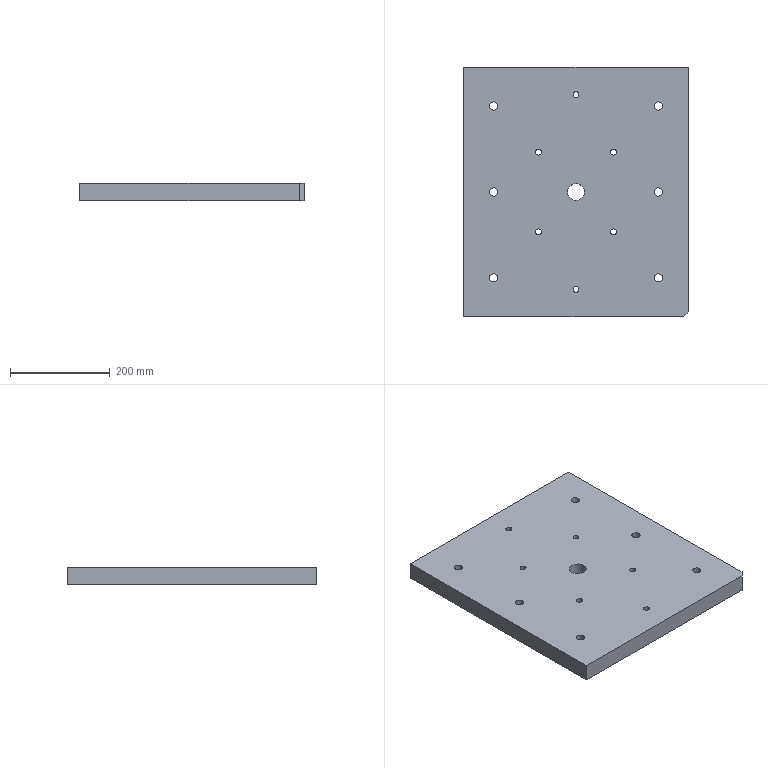Part | STEP file | SL2-MOLD_id750_xmt_txt | 1 solid | 45 faces | box 450 x 500 x 35 mm | volume 7734159 mm3 | cylinder 25 | plane 19 | cone 1 | commonest cylinder face diameters 12 x6 16.5 x6 18 x6 25 x6 34 x1
STEP:
#1=CARTESIAN_POINT('',(225.,340.,-244.));
#2=VERTEX_POINT('',#1);
#3=CARTESIAN_POINT('',(-225.,340.,-244.));
#4=VERTEX_POINT('',#3);
#5=CARTESIAN_POINT('',(0.,340.,-244.));
#6=DIRECTION('',(-1.,0.,0.));
#7=VECTOR('',#6,1.);
#8=LINE('',#5,#7);
#9=EDGE_CURVE('',#2,#4,#8,.T.);
#10=ORIENTED_EDGE('',*,*,#9,.F.);
#11=CARTESIAN_POINT('',(225.,340.,-279.));
#12=VERTEX_POINT('',#11);
#13=CARTESIAN_POINT('',(225.,340.,186.));
#14=DIRECTION('',(0.,0.,1.));
#15=VECTOR('',#14,1.);
#16=LINE('',#13,#15);
#17=EDGE_CURVE('',#12,#2,#16,.T.);
#18=ORIENTED_EDGE('',*,*,#17,.F.);
#19=CARTESIAN_POINT('',(-225.,340.,-279.));
#20=VERTEX_POINT('',#19);
#21=CARTESIAN_POINT('',(0.,340.,-279.));
#22=DIRECTION('',(-1.,0.,0.));
#23=VECTOR('',#22,1.);
#24=LINE('',#21,#23);
#25=EDGE_CURVE('',#12,#20,#24,.T.);
#26=ORIENTED_EDGE('',*,*,#25,.T.);
#27=CARTESIAN_POINT('',(-225.,340.,-279.));
#28=DIRECTION('',(0.,0.,1.));
#29=VECTOR('',#28,1.);
#30=LINE('',#27,#29);
#31=EDGE_CURVE('',#20,#4,#30,.T.);
#32=ORIENTED_EDGE('',*,*,#31,.T.);
#33=EDGE_LOOP('',(#10,#18,#26,#32));
#34=FACE_OUTER_BOUND('',#33,.T.);
#35=CARTESIAN_POINT('',(0.,340.,-279.));
#36=DIRECTION('',(0.,1.,0.));
#37=DIRECTION('',(0.,0.,1.));
#38=AXIS2_PLACEMENT_3D('',#35,#36,#37);
#39=PLANE('',#38);
#40=ADVANCED_FACE('',(#34),#39,.T.);
#41=CARTESIAN_POINT('',(225.,-150.,-244.));
#42=VERTEX_POINT('',#41);
#43=CARTESIAN_POINT('',(225.,0.,-244.));
#44=DIRECTION('',(0.,1.,0.));
#45=VECTOR('',#44,1.);
#46=LINE('',#43,#45);
#47=EDGE_CURVE('',#42,#2,#46,.T.);
#48=ORIENTED_EDGE('',*,*,#47,.F.);
#49=CARTESIAN_POINT('',(225.,-150.,-279.));
#50=VERTEX_POINT('',#49);
#51=CARTESIAN_POINT('',(225.,-150.,186.));
#52=DIRECTION('',(0.,0.,-1.));
#53=VECTOR('',#52,1.);
#54=LINE('',#51,#53);
#55=EDGE_CURVE('',#42,#50,#54,.T.);
#56=ORIENTED_EDGE('',*,*,#55,.T.);
#57=CARTESIAN_POINT('',(225.,0.,-279.));
#58=DIRECTION('',(0.,1.,0.));
#59=VECTOR('',#58,1.);
#60=LINE('',#57,#59);
#61=EDGE_CURVE('',#50,#12,#60,.T.);
#62=ORIENTED_EDGE('',*,*,#61,.T.);
#63=ORIENTED_EDGE('',*,*,#17,.T.);
#64=EDGE_LOOP('',(#48,#56,#62,#63));
#65=FACE_OUTER_BOUND('',#64,.T.);
#66=CARTESIAN_POINT('',(225.,-110.,186.));
#67=DIRECTION('',(1.,0.,0.));
#68=DIRECTION('',(0.,0.,-1.));
#69=AXIS2_PLACEMENT_3D('',#66,#67,#68);
#70=PLANE('',#69);
#71=ADVANCED_FACE('',(#65),#70,.T.);
#72=CARTESIAN_POINT('',(-225.,-160.,-279.));
#73=VERTEX_POINT('',#72);
#74=CARTESIAN_POINT('',(215.,-160.,-279.));
#75=VERTEX_POINT('',#74);
#76=CARTESIAN_POINT('',(0.,-160.,-279.));
#77=DIRECTION('',(1.,0.,0.));
#78=VECTOR('',#77,1.);
#79=LINE('',#76,#78);
#80=EDGE_CURVE('',#73,#75,#79,.T.);
#81=ORIENTED_EDGE('',*,*,#80,.T.);
#82=CARTESIAN_POINT('',(215.,-160.,-244.));
#83=VERTEX_POINT('',#82);
#84=CARTESIAN_POINT('',(215.,-160.,-279.));
#85=DIRECTION('',(0.,0.,1.));
#86=VECTOR('',#85,1.);
#87=LINE('',#84,#86);
#88=EDGE_CURVE('',#75,#83,#87,.T.);
#89=ORIENTED_EDGE('',*,*,#88,.T.);
#90=CARTESIAN_POINT('',(-225.,-160.,-244.));
#91=VERTEX_POINT('',#90);
#92=CARTESIAN_POINT('',(0.,-160.,-244.));
#93=DIRECTION('',(1.,0.,0.));
#94=VECTOR('',#93,1.);
#95=LINE('',#92,#94);
#96=EDGE_CURVE('',#91,#83,#95,.T.);
#97=ORIENTED_EDGE('',*,*,#96,.F.);
#98=CARTESIAN_POINT('',(-225.,-160.,186.));
#99=DIRECTION('',(0.,0.,1.));
#100=VECTOR('',#99,1.);
#101=LINE('',#98,#100);
#102=EDGE_CURVE('',#73,#91,#101,.T.);
#103=ORIENTED_EDGE('',*,*,#102,.F.);
#104=EDGE_LOOP('',(#81,#89,#97,#103));
#105=FACE_OUTER_BOUND('',#104,.T.);
#106=CARTESIAN_POINT('',(0.,-160.,-279.));
#107=DIRECTION('',(0.,-1.,0.));
#108=DIRECTION('',(0.,0.,-1.));
#109=AXIS2_PLACEMENT_3D('',#106,#107,#108);
#110=PLANE('',#109);
#111=ADVANCED_FACE('',(#105),#110,.T.);
#112=CARTESIAN_POINT('',(-225.,0.,-244.));
#113=DIRECTION('',(0.,-1.,0.));
#114=VECTOR('',#113,1.);
#115=LINE('',#112,#114);
#116=EDGE_CURVE('',#4,#91,#115,.T.);
#117=ORIENTED_EDGE('',*,*,#116,.F.);
#118=ORIENTED_EDGE('',*,*,#31,.F.);
#119=CARTESIAN_POINT('',(-225.,0.,-279.));
#120=DIRECTION('',(0.,-1.,0.));
#121=VECTOR('',#120,1.);
#122=LINE('',#119,#121);
#123=EDGE_CURVE('',#20,#73,#122,.T.);
#124=ORIENTED_EDGE('',*,*,#123,.T.);
#125=ORIENTED_EDGE('',*,*,#102,.T.);
#126=EDGE_LOOP('',(#117,#118,#124,#125));
#127=FACE_OUTER_BOUND('',#126,.T.);
#128=CARTESIAN_POINT('',(-225.,-4.582,186.));
#129=DIRECTION('',(-1.,0.,0.));
#130=DIRECTION('',(0.,0.,1.));
#131=AXIS2_PLACEMENT_3D('',#128,#129,#130);
#132=PLANE('',#131);
#133=ADVANCED_FACE('',(#127),#132,.T.);
#134=CARTESIAN_POINT('',(9.,285.,-279.));
#135=VERTEX_POINT('',#134);
#136=CARTESIAN_POINT('',(0.,285.,-279.));
#137=DIRECTION('',(0.,0.,1.));
#138=DIRECTION('',(1.,0.,0.));
#139=AXIS2_PLACEMENT_3D('',#136,#137,#138);
#140=CIRCLE('',#139,9.);
#141=EDGE_CURVE('',#135,#135,#140,.T.);
#142=ORIENTED_EDGE('',*,*,#141,.T.);
#143=EDGE_LOOP('',(#142));
#144=FACE_BOUND('',#143,.T.);
#145=CARTESIAN_POINT('',(84.,170.,-279.));
#146=VERTEX_POINT('',#145);
#147=CARTESIAN_POINT('',(75.,170.,-279.));
#148=DIRECTION('',(0.,0.,1.));
#149=DIRECTION('',(1.,0.,0.));
#150=AXIS2_PLACEMENT_3D('',#147,#148,#149);
#151=CIRCLE('',#150,9.);
#152=EDGE_CURVE('',#146,#146,#151,.T.);
#153=ORIENTED_EDGE('',*,*,#152,.T.);
#154=EDGE_LOOP('',(#153));
#155=FACE_BOUND('',#154,.T.);
#156=CARTESIAN_POINT('',(-66.,170.,-279.));
#157=VERTEX_POINT('',#156);
#158=CARTESIAN_POINT('',(-75.,170.,-279.));
#159=DIRECTION('',(0.,0.,1.));
#160=DIRECTION('',(1.,0.,0.));
#161=AXIS2_PLACEMENT_3D('',#158,#159,#160);
#162=CIRCLE('',#161,9.);
#163=EDGE_CURVE('',#157,#157,#162,.T.);
#164=ORIENTED_EDGE('',*,*,#163,.T.);
#165=EDGE_LOOP('',(#164));
#166=FACE_BOUND('',#165,.T.);
#167=CARTESIAN_POINT('',(-66.,10.,-279.));
#168=VERTEX_POINT('',#167);
#169=CARTESIAN_POINT('',(-75.,10.,-279.));
#170=DIRECTION('',(0.,0.,1.));
#171=DIRECTION('',(1.,0.,0.));
#172=AXIS2_PLACEMENT_3D('',#169,#170,#171);
#173=CIRCLE('',#172,9.);
#174=EDGE_CURVE('',#168,#168,#173,.T.);
#175=ORIENTED_EDGE('',*,*,#174,.T.);
#176=EDGE_LOOP('',(#175));
#177=FACE_BOUND('',#176,.T.);
#178=CARTESIAN_POINT('',(9.,-105.,-279.));
#179=VERTEX_POINT('',#178);
#180=CARTESIAN_POINT('',(0.,-105.,-279.));
#181=DIRECTION('',(0.,0.,1.));
#182=DIRECTION('',(1.,0.,0.));
#183=AXIS2_PLACEMENT_3D('',#180,#181,#182);
#184=CIRCLE('',#183,9.);
#185=EDGE_CURVE('',#179,#179,#184,.T.);
#186=ORIENTED_EDGE('',*,*,#185,.T.);
#187=EDGE_LOOP('',(#186));
#188=FACE_BOUND('',#187,.T.);
#189=CARTESIAN_POINT('',(84.,10.,-279.));
#190=VERTEX_POINT('',#189);
#191=CARTESIAN_POINT('',(75.,10.,-279.));
#192=DIRECTION('',(0.,0.,1.));
#193=DIRECTION('',(1.,0.,0.));
#194=AXIS2_PLACEMENT_3D('',#191,#192,#193);
#195=CIRCLE('',#194,9.);
#196=EDGE_CURVE('',#190,#190,#195,.T.);
#197=ORIENTED_EDGE('',*,*,#196,.T.);
#198=EDGE_LOOP('',(#197));
#199=FACE_BOUND('',#198,.T.);
#200=CARTESIAN_POINT('',(19.,90.,-279.));
#201=VERTEX_POINT('',#200);
#202=CARTESIAN_POINT('',(0.,90.,-279.));
#203=DIRECTION('',(0.,0.,1.));
#204=DIRECTION('',(1.,0.,0.));
#205=AXIS2_PLACEMENT_3D('',#202,#203,#204);
#206=CIRCLE('',#205,19.);
#207=EDGE_CURVE('',#201,#201,#206,.T.);
#208=ORIENTED_EDGE('',*,*,#207,.T.);
#209=EDGE_LOOP('',(#208));
#210=FACE_BOUND('',#209,.T.);
#211=CARTESIAN_POINT('',(177.5,-82.,-279.));
#212=VERTEX_POINT('',#211);
#213=CARTESIAN_POINT('',(165.,-82.,-279.));
#214=DIRECTION('',(0.,0.,-1.));
#215=DIRECTION('',(1.,0.,0.));
#216=AXIS2_PLACEMENT_3D('',#213,#214,#215);
#217=CIRCLE('',#216,12.5);
#218=EDGE_CURVE('',#212,#212,#217,.T.);
#219=ORIENTED_EDGE('',*,*,#218,.F.);
#220=EDGE_LOOP('',(#219));
#221=FACE_BOUND('',#220,.T.);
#222=CARTESIAN_POINT('',(177.5,90.,-279.));
#223=VERTEX_POINT('',#222);
#224=CARTESIAN_POINT('',(165.,90.,-279.));
#225=DIRECTION('',(0.,0.,-1.));
#226=DIRECTION('',(1.,0.,0.));
#227=AXIS2_PLACEMENT_3D('',#224,#225,#226);
#228=CIRCLE('',#227,12.5);
#229=EDGE_CURVE('',#223,#223,#228,.T.);
#230=ORIENTED_EDGE('',*,*,#229,.F.);
#231=EDGE_LOOP('',(#230));
#232=FACE_BOUND('',#231,.T.);
#233=CARTESIAN_POINT('',(-152.5,-82.,-279.));
#234=VERTEX_POINT('',#233);
#235=CARTESIAN_POINT('',(-165.,-82.,-279.));
#236=DIRECTION('',(0.,0.,-1.));
#237=DIRECTION('',(1.,0.,0.));
#238=AXIS2_PLACEMENT_3D('',#235,#236,#237);
#239=CIRCLE('',#238,12.5);
#240=EDGE_CURVE('',#234,#234,#239,.T.);
#241=ORIENTED_EDGE('',*,*,#240,.F.);
#242=EDGE_LOOP('',(#241));
#243=FACE_BOUND('',#242,.T.);
#244=CARTESIAN_POINT('',(-152.5,90.,-279.));
#245=VERTEX_POINT('',#244);
#246=CARTESIAN_POINT('',(-165.,90.,-279.));
#247=DIRECTION('',(0.,0.,-1.));
#248=DIRECTION('',(1.,0.,0.));
#249=AXIS2_PLACEMENT_3D('',#246,#247,#248);
#250=CIRCLE('',#249,12.5);
#251=EDGE_CURVE('',#245,#245,#250,.T.);
#252=ORIENTED_EDGE('',*,*,#251,.F.);
#253=EDGE_LOOP('',(#252));
#254=FACE_BOUND('',#253,.T.);
#255=CARTESIAN_POINT('',(-152.5,262.,-279.));
#256=VERTEX_POINT('',#255);
#257=CARTESIAN_POINT('',(-165.,262.,-279.));
#258=DIRECTION('',(0.,0.,-1.));
#259=DIRECTION('',(1.,0.,0.));
#260=AXIS2_PLACEMENT_3D('',#257,#258,#259);
#261=CIRCLE('',#260,12.5);
#262=EDGE_CURVE('',#256,#256,#261,.T.);
#263=ORIENTED_EDGE('',*,*,#262,.F.);
#264=EDGE_LOOP('',(#263));
#265=FACE_BOUND('',#264,.T.);
#266=CARTESIAN_POINT('',(177.5,262.,-279.));
#267=VERTEX_POINT('',#266);
#268=CARTESIAN_POINT('',(165.,262.,-279.));
#269=DIRECTION('',(0.,0.,-1.));
#270=DIRECTION('',(1.,0.,0.));
#271=AXIS2_PLACEMENT_3D('',#268,#269,#270);
#272=CIRCLE('',#271,12.5);
#273=EDGE_CURVE('',#267,#267,#272,.T.);
#274=ORIENTED_EDGE('',*,*,#273,.F.);
#275=EDGE_LOOP('',(#274));
#276=FACE_BOUND('',#275,.T.);
#277=ORIENTED_EDGE('',*,*,#61,.F.);
#278=CARTESIAN_POINT('',(215.,-160.,-279.));
#279=DIRECTION('',(-0.7071,-0.7071,0.));
#280=VECTOR('',#279,1.);
#281=LINE('',#278,#280);
#282=EDGE_CURVE('',#50,#75,#281,.T.);
#283=ORIENTED_EDGE('',*,*,#282,.T.);
#284=ORIENTED_EDGE('',*,*,#80,.F.);
#285=ORIENTED_EDGE('',*,*,#123,.F.);
#286=ORIENTED_EDGE('',*,*,#25,.F.);
#287=EDGE_LOOP('',(#277,#283,#284,#285,#286));
#288=FACE_BOUND('',#287,.T.);
#289=CARTESIAN_POINT('',(0.,0.,-279.));
#290=DIRECTION('',(0.,0.,1.));
#291=DIRECTION('',(1.,0.,0.));
#292=AXIS2_PLACEMENT_3D('',#289,#290,#291);
#293=PLANE('',#292);
#294=ADVANCED_FACE('',(#144,#155,#166,#177,#188,#199,#210,#221,#232,#243,#254,#265,#276,#288),#293,.F.);
#295=CARTESIAN_POINT('',(-69.,10.,-244.));
#296=VERTEX_POINT('',#295);
#297=CARTESIAN_POINT('',(-75.,10.,-244.));
#298=DIRECTION('',(0.,0.,-1.));
#299=DIRECTION('',(1.,0.,0.));
#300=AXIS2_PLACEMENT_3D('',#297,#298,#299);
#301=CIRCLE('',#300,6.);
#302=EDGE_CURVE('',#296,#296,#301,.T.);
#303=ORIENTED_EDGE('',*,*,#302,.T.);
#304=EDGE_LOOP('',(#303));
#305=FACE_BOUND('',#304,.T.);
#306=CARTESIAN_POINT('',(-69.,170.,-244.));
#307=VERTEX_POINT('',#306);
#308=CARTESIAN_POINT('',(-75.,170.,-244.));
#309=DIRECTION('',(0.,0.,-1.));
#310=DIRECTION('',(1.,0.,0.));
#311=AXIS2_PLACEMENT_3D('',#308,#309,#310);
#312=CIRCLE('',#311,6.);
#313=EDGE_CURVE('',#307,#307,#312,.T.);
#314=ORIENTED_EDGE('',*,*,#313,.T.);
#315=EDGE_LOOP('',(#314));
#316=FACE_BOUND('',#315,.T.);
#317=CARTESIAN_POINT('',(6.,285.,-244.));
#318=VERTEX_POINT('',#317);
#319=CARTESIAN_POINT('',(0.,285.,-244.));
#320=DIRECTION('',(0.,0.,-1.));
#321=DIRECTION('',(1.,0.,0.));
#322=AXIS2_PLACEMENT_3D('',#319,#320,#321);
#323=CIRCLE('',#322,6.);
#324=EDGE_CURVE('',#318,#318,#323,.T.);
#325=ORIENTED_EDGE('',*,*,#324,.T.);
#326=EDGE_LOOP('',(#325));
#327=FACE_BOUND('',#326,.T.);
#328=CARTESIAN_POINT('',(81.,170.,-244.));
#329=VERTEX_POINT('',#328);
#330=CARTESIAN_POINT('',(75.,170.,-244.));
#331=DIRECTION('',(0.,0.,-1.));
#332=DIRECTION('',(1.,0.,0.));
#333=AXIS2_PLACEMENT_3D('',#330,#331,#332);
#334=CIRCLE('',#333,6.);
#335=EDGE_CURVE('',#329,#329,#334,.T.);
#336=ORIENTED_EDGE('',*,*,#335,.T.);
#337=EDGE_LOOP('',(#336));
#338=FACE_BOUND('',#337,.T.);
#339=CARTESIAN_POINT('',(81.,10.,-244.));
#340=VERTEX_POINT('',#339);
#341=CARTESIAN_POINT('',(75.,10.,-244.));
#342=DIRECTION('',(0.,0.,-1.));
#343=DIRECTION('',(1.,0.,0.));
#344=AXIS2_PLACEMENT_3D('',#341,#342,#343);
#345=CIRCLE('',#344,6.);
#346=EDGE_CURVE('',#340,#340,#345,.T.);
#347=ORIENTED_EDGE('',*,*,#346,.T.);
#348=EDGE_LOOP('',(#347));
#349=FACE_BOUND('',#348,.T.);
#350=CARTESIAN_POINT('',(6.,-105.,-244.));
#351=VERTEX_POINT('',#350);
#352=CARTESIAN_POINT('',(0.,-105.,-244.));
#353=DIRECTION('',(0.,0.,-1.));
#354=DIRECTION('',(1.,0.,0.));
#355=AXIS2_PLACEMENT_3D('',#352,#353,#354);
#356=CIRCLE('',#355,6.);
#357=EDGE_CURVE('',#351,#351,#356,.T.);
#358=ORIENTED_EDGE('',*,*,#357,.T.);
#359=EDGE_LOOP('',(#358));
#360=FACE_BOUND('',#359,.T.);
#361=CARTESIAN_POINT('',(17.,90.,-244.));
#362=VERTEX_POINT('',#361);
#363=CARTESIAN_POINT('',(0.,90.,-244.));
#364=DIRECTION('',(0.,0.,1.));
#365=DIRECTION('',(1.,0.,0.));
#366=AXIS2_PLACEMENT_3D('',#363,#364,#365);
#367=CIRCLE('',#366,17.);
#368=EDGE_CURVE('',#362,#362,#367,.T.);
#369=ORIENTED_EDGE('',*,*,#368,.F.);
#370=EDGE_LOOP('',(#369));
#371=FACE_BOUND('',#370,.T.);
#372=CARTESIAN_POINT('',(-156.75,262.,-244.));
#373=VERTEX_POINT('',#372);
#374=CARTESIAN_POINT('',(-165.,262.,-244.));
#375=DIRECTION('',(0.,0.,1.));
#376=DIRECTION('',(1.,0.,0.));
#377=AXIS2_PLACEMENT_3D('',#374,#375,#376);
#378=CIRCLE('',#377,8.25);
#379=EDGE_CURVE('',#373,#373,#378,.T.);
#380=ORIENTED_EDGE('',*,*,#379,.F.);
#381=EDGE_LOOP('',(#380));
#382=FACE_BOUND('',#381,.T.);
#383=CARTESIAN_POINT('',(-156.75,90.,-244.));
#384=VERTEX_POINT('',#383);
#385=CARTESIAN_POINT('',(-165.,90.,-244.));
#386=DIRECTION('',(0.,0.,1.));
#387=DIRECTION('',(1.,0.,0.));
#388=AXIS2_PLACEMENT_3D('',#385,#386,#387);
#389=CIRCLE('',#388,8.25);
#390=EDGE_CURVE('',#384,#384,#389,.T.);
#391=ORIENTED_EDGE('',*,*,#390,.F.);
#392=EDGE_LOOP('',(#391));
#393=FACE_BOUND('',#392,.T.);
#394=CARTESIAN_POINT('',(-156.75,-82.,-244.));
#395=VERTEX_POINT('',#394);
#396=CARTESIAN_POINT('',(-165.,-82.,-244.));
#397=DIRECTION('',(0.,0.,1.));
#398=DIRECTION('',(1.,0.,0.));
#399=AXIS2_PLACEMENT_3D('',#396,#397,#398);
#400=CIRCLE('',#399,8.25);
#401=EDGE_CURVE('',#395,#395,#400,.T.);
#402=ORIENTED_EDGE('',*,*,#401,.F.);
#403=EDGE_LOOP('',(#402));
#404=FACE_BOUND('',#403,.T.);
#405=CARTESIAN_POINT('',(173.25,-82.,-244.));
#406=VERTEX_POINT('',#405);
#407=CARTESIAN_POINT('',(165.,-82.,-244.));
#408=DIRECTION('',(0.,0.,1.));
#409=DIRECTION('',(1.,0.,0.));
#410=AXIS2_PLACEMENT_3D('',#407,#408,#409);
#411=CIRCLE('',#410,8.25);
#412=EDGE_CURVE('',#406,#406,#411,.T.);
#413=ORIENTED_EDGE('',*,*,#412,.F.);
#414=EDGE_LOOP('',(#413));
#415=FACE_BOUND('',#414,.T.);
#416=CARTESIAN_POINT('',(173.25,90.,-244.));
#417=VERTEX_POINT('',#416);
#418=CARTESIAN_POINT('',(165.,90.,-244.));
#419=DIRECTION('',(0.,0.,1.));
#420=DIRECTION('',(1.,0.,0.));
#421=AXIS2_PLACEMENT_3D('',#418,#419,#420);
#422=CIRCLE('',#421,8.25);
#423=EDGE_CURVE('',#417,#417,#422,.T.);
#424=ORIENTED_EDGE('',*,*,#423,.F.);
#425=EDGE_LOOP('',(#424));
#426=FACE_BOUND('',#425,.T.);
#427=CARTESIAN_POINT('',(173.25,262.,-244.));
#428=VERTEX_POINT('',#427);
#429=CARTESIAN_POINT('',(165.,262.,-244.));
#430=DIRECTION('',(0.,0.,1.));
#431=DIRECTION('',(1.,0.,0.));
#432=AXIS2_PLACEMENT_3D('',#429,#430,#431);
#433=CIRCLE('',#432,8.25);
#434=EDGE_CURVE('',#428,#428,#433,.T.);
#435=ORIENTED_EDGE('',*,*,#434,.F.);
#436=EDGE_LOOP('',(#435));
#437=FACE_BOUND('',#436,.T.);
#438=ORIENTED_EDGE('',*,*,#96,.T.);
#439=CARTESIAN_POINT('',(187.5,-187.5,-244.));
#440=DIRECTION('',(0.7071,0.7071,0.));
#441=VECTOR('',#440,1.);
#442=LINE('',#439,#441);
#443=EDGE_CURVE('',#83,#42,#442,.T.);
#444=ORIENTED_EDGE('',*,*,#443,.T.);
#445=ORIENTED_EDGE('',*,*,#47,.T.);
#446=ORIENTED_EDGE('',*,*,#9,.T.);
#447=ORIENTED_EDGE('',*,*,#116,.T.);
#448=EDGE_LOOP('',(#438,#444,#445,#446,#447));
#449=FACE_BOUND('',#448,.T.);
#450=CARTESIAN_POINT('',(0.,0.,-244.));
#451=DIRECTION('',(0.,0.,1.));
#452=DIRECTION('',(1.,0.,0.));
#453=AXIS2_PLACEMENT_3D('',#450,#451,#452);
#454=PLANE('',#453);
#455=ADVANCED_FACE('',(#305,#316,#327,#338,#349,#360,#371,#382,#393,#404,#415,#426,#437,#449),#454,.T.);
#456=ORIENTED_EDGE('',*,*,#282,.F.);
#457=ORIENTED_EDGE('',*,*,#55,.F.);
#458=ORIENTED_EDGE('',*,*,#443,.F.);
#459=ORIENTED_EDGE('',*,*,#88,.F.);
#460=EDGE_LOOP('',(#456,#457,#458,#459));
#461=FACE_OUTER_BOUND('',#460,.T.);
#462=CARTESIAN_POINT('',(215.,-160.,-279.));
#463=DIRECTION('',(-0.7071,0.7071,0.));
#464=DIRECTION('',(0.,0.,1.));
#465=AXIS2_PLACEMENT_3D('',#462,#463,#464);
#466=PLANE('',#465);
#467=ADVANCED_FACE('',(#461),#466,.F.);
#468=CARTESIAN_POINT('',(152.5,262.,-262.));
#469=VERTEX_POINT('',#468);
#470=CARTESIAN_POINT('',(165.,262.,-262.));
#471=DIRECTION('',(0.,0.,1.));
#472=DIRECTION('',(-1.,0.,0.));
#473=AXIS2_PLACEMENT_3D('',#470,#471,#472);
#474=CIRCLE('',#473,12.5);
#475=EDGE_CURVE('',#469,#469,#474,.T.);
#476=ORIENTED_EDGE('',*,*,#475,.T.);
#477=EDGE_LOOP('',(#476));
#478=FACE_BOUND('',#477,.T.);
#479=ORIENTED_EDGE('',*,*,#273,.T.);
#480=EDGE_LOOP('',(#479));
#481=FACE_BOUND('',#480,.T.);
#482=CARTESIAN_POINT('',(165.,262.,-292.));
#483=DIRECTION('',(0.,0.,1.));
#484=DIRECTION('',(1.,0.,0.));
#485=AXIS2_PLACEMENT_3D('',#482,#483,#484);
#486=CYLINDRICAL_SURFACE('',#485,12.5);
#487=ADVANCED_FACE('',(#478,#481),#486,.F.);
#488=CARTESIAN_POINT('',(156.75,262.,-262.));
#489=VERTEX_POINT('',#488);
#490=CARTESIAN_POINT('',(165.,262.,-262.));
#491=DIRECTION('',(0.,0.,-1.));
#492=DIRECTION('',(-1.,0.,0.));
#493=AXIS2_PLACEMENT_3D('',#490,#491,#492);
#494=CIRCLE('',#493,8.25);
#495=EDGE_CURVE('',#489,#489,#494,.T.);
#496=ORIENTED_EDGE('',*,*,#495,.F.);
#497=EDGE_LOOP('',(#496));
#498=FACE_BOUND('',#497,.T.);
#499=ORIENTED_EDGE('',*,*,#475,.F.);
#500=EDGE_LOOP('',(#499));
#501=FACE_BOUND('',#500,.T.);
#502=CARTESIAN_POINT('',(165.,262.,-262.));
#503=DIRECTION('',(0.,0.,-1.));
#504=DIRECTION('',(-1.,0.,0.));
#505=AXIS2_PLACEMENT_3D('',#502,#503,#504);
#506=PLANE('',#505);
#507=ADVANCED_FACE('',(#498,#501),#506,.T.);
#508=CARTESIAN_POINT('',(-177.5,262.,-262.));
#509=VERTEX_POINT('',#508);
#510=CARTESIAN_POINT('',(-165.,262.,-262.));
#511=DIRECTION('',(0.,0.,1.));
#512=DIRECTION('',(-1.,0.,0.));
#513=AXIS2_PLACEMENT_3D('',#510,#511,#512);
#514=CIRCLE('',#513,12.5);
#515=EDGE_CURVE('',#509,#509,#514,.T.);
#516=ORIENTED_EDGE('',*,*,#515,.T.);
#517=EDGE_LOOP('',(#516));
#518=FACE_BOUND('',#517,.T.);
#519=ORIENTED_EDGE('',*,*,#262,.T.);
#520=EDGE_LOOP('',(#519));
#521=FACE_BOUND('',#520,.T.);
#522=CARTESIAN_POINT('',(-165.,262.,-292.));
#523=DIRECTION('',(0.,0.,1.));
#524=DIRECTION('',(1.,0.,0.));
#525=AXIS2_PLACEMENT_3D('',#522,#523,#524);
#526=CYLINDRICAL_SURFACE('',#525,12.5);
#527=ADVANCED_FACE('',(#518,#521),#526,.F.);
#528=CARTESIAN_POINT('',(-173.25,262.,-262.));
#529=VERTEX_POINT('',#528);
#530=CARTESIAN_POINT('',(-165.,262.,-262.));
#531=DIRECTION('',(0.,0.,-1.));
#532=DIRECTION('',(-1.,0.,0.));
#533=AXIS2_PLACEMENT_3D('',#530,#531,#532);
#534=CIRCLE('',#533,8.25);
#535=EDGE_CURVE('',#529,#529,#534,.T.);
#536=ORIENTED_EDGE('',*,*,#535,.F.);
#537=EDGE_LOOP('',(#536));
#538=FACE_BOUND('',#537,.T.);
#539=ORIENTED_EDGE('',*,*,#515,.F.);
#540=EDGE_LOOP('',(#539));
#541=FACE_BOUND('',#540,.T.);
#542=CARTESIAN_POINT('',(-165.,262.,-262.));
#543=DIRECTION('',(0.,0.,-1.));
#544=DIRECTION('',(-1.,0.,0.));
#545=AXIS2_PLACEMENT_3D('',#542,#543,#544);
#546=PLANE('',#545);
#547=ADVANCED_FACE('',(#538,#541),#546,.T.);
#548=CARTESIAN_POINT('',(-177.5,90.,-262.));
#549=VERTEX_POINT('',#548);
#550=CARTESIAN_POINT('',(-165.,90.,-262.));
#551=DIRECTION('',(0.,0.,1.));
#552=DIRECTION('',(-1.,0.,0.));
#553=AXIS2_PLACEMENT_3D('',#550,#551,#552);
#554=CIRCLE('',#553,12.5);
#555=EDGE_CURVE('',#549,#549,#554,.T.);
#556=ORIENTED_EDGE('',*,*,#555,.T.);
#557=EDGE_LOOP('',(#556));
#558=FACE_BOUND('',#557,.T.);
#559=ORIENTED_EDGE('',*,*,#251,.T.);
#560=EDGE_LOOP('',(#559));
#561=FACE_BOUND('',#560,.T.);
#562=CARTESIAN_POINT('',(-165.,90.,-292.));
#563=DIRECTION('',(0.,0.,1.));
#564=DIRECTION('',(1.,0.,0.));
#565=AXIS2_PLACEMENT_3D('',#562,#563,#564);
#566=CYLINDRICAL_SURFACE('',#565,12.5);
#567=ADVANCED_FACE('',(#558,#561),#566,.F.);
#568=CARTESIAN_POINT('',(-173.25,90.,-262.));
#569=VERTEX_POINT('',#568);
#570=CARTESIAN_POINT('',(-165.,90.,-262.));
#571=DIRECTION('',(0.,0.,-1.));
#572=DIRECTION('',(-1.,0.,0.));
#573=AXIS2_PLACEMENT_3D('',#570,#571,#572);
#574=CIRCLE('',#573,8.25);
#575=EDGE_CURVE('',#569,#569,#574,.T.);
#576=ORIENTED_EDGE('',*,*,#575,.F.);
#577=EDGE_LOOP('',(#576));
#578=FACE_BOUND('',#577,.T.);
#579=ORIENTED_EDGE('',*,*,#555,.F.);
#580=EDGE_LOOP('',(#579));
#581=FACE_BOUND('',#580,.T.);
#582=CARTESIAN_POINT('',(-165.,90.,-262.));
#583=DIRECTION('',(0.,0.,-1.));
#584=DIRECTION('',(-1.,0.,0.));
#585=AXIS2_PLACEMENT_3D('',#582,#583,#584);
#586=PLANE('',#585);
#587=ADVANCED_FACE('',(#578,#581),#586,.T.);
#588=CARTESIAN_POINT('',(-177.5,-82.,-262.));
#589=VERTEX_POINT('',#588);
#590=CARTESIAN_POINT('',(-165.,-82.,-262.));
#591=DIRECTION('',(0.,0.,1.));
#592=DIRECTION('',(-1.,0.,0.));
#593=AXIS2_PLACEMENT_3D('',#590,#591,#592);
#594=CIRCLE('',#593,12.5);
#595=EDGE_CURVE('',#589,#589,#594,.T.);
#596=ORIENTED_EDGE('',*,*,#595,.T.);
#597=EDGE_LOOP('',(#596));
#598=FACE_BOUND('',#597,.T.);
#599=ORIENTED_EDGE('',*,*,#240,.T.);
#600=EDGE_LOOP('',(#599));
#601=FACE_BOUND('',#600,.T.);
#602=CARTESIAN_POINT('',(-165.,-82.,-292.));
#603=DIRECTION('',(0.,0.,1.));
#604=DIRECTION('',(1.,0.,0.));
#605=AXIS2_PLACEMENT_3D('',#602,#603,#604);
#606=CYLINDRICAL_SURFACE('',#605,12.5);
#607=ADVANCED_FACE('',(#598,#601),#606,.F.);
#608=CARTESIAN_POINT('',(-173.25,-82.,-262.));
#609=VERTEX_POINT('',#608);
#610=CARTESIAN_POINT('',(-165.,-82.,-262.));
#611=DIRECTION('',(0.,0.,-1.));
#612=DIRECTION('',(-1.,0.,0.));
#613=AXIS2_PLACEMENT_3D('',#610,#611,#612);
#614=CIRCLE('',#613,8.25);
#615=EDGE_CURVE('',#609,#609,#614,.T.);
#616=ORIENTED_EDGE('',*,*,#615,.F.);
#617=EDGE_LOOP('',(#616));
#618=FACE_BOUND('',#617,.T.);
#619=ORIENTED_EDGE('',*,*,#595,.F.);
#620=EDGE_LOOP('',(#619));
#621=FACE_BOUND('',#620,.T.);
#622=CARTESIAN_POINT('',(-165.,-82.,-262.));
#623=DIRECTION('',(0.,0.,-1.));
#624=DIRECTION('',(-1.,0.,0.));
#625=AXIS2_PLACEMENT_3D('',#622,#623,#624);
#626=PLANE('',#625);
#627=ADVANCED_FACE('',(#618,#621),#626,.T.);
#628=CARTESIAN_POINT('',(152.5,90.,-262.));
#629=VERTEX_POINT('',#628);
#630=CARTESIAN_POINT('',(165.,90.,-262.));
#631=DIRECTION('',(0.,0.,1.));
#632=DIRECTION('',(-1.,0.,0.));
#633=AXIS2_PLACEMENT_3D('',#630,#631,#632);
#634=CIRCLE('',#633,12.5);
#635=EDGE_CURVE('',#629,#629,#634,.T.);
#636=ORIENTED_EDGE('',*,*,#635,.T.);
#637=EDGE_LOOP('',(#636));
#638=FACE_BOUND('',#637,.T.);
#639=ORIENTED_EDGE('',*,*,#229,.T.);
#640=EDGE_LOOP('',(#639));
#641=FACE_BOUND('',#640,.T.);
#642=CARTESIAN_POINT('',(165.,90.,-292.));
#643=DIRECTION('',(0.,0.,1.));
#644=DIRECTION('',(1.,0.,0.));
#645=AXIS2_PLACEMENT_3D('',#642,#643,#644);
#646=CYLINDRICAL_SURFACE('',#645,12.5);
#647=ADVANCED_FACE('',(#638,#641),#646,.F.);
#648=CARTESIAN_POINT('',(156.75,90.,-262.));
#649=VERTEX_POINT('',#648);
#650=CARTESIAN_POINT('',(165.,90.,-262.));
#651=DIRECTION('',(0.,0.,-1.));
#652=DIRECTION('',(-1.,0.,0.));
#653=AXIS2_PLACEMENT_3D('',#650,#651,#652);
#654=CIRCLE('',#653,8.25);
#655=EDGE_CURVE('',#649,#649,#654,.T.);
#656=ORIENTED_EDGE('',*,*,#655,.F.);
#657=EDGE_LOOP('',(#656));
#658=FACE_BOUND('',#657,.T.);
#659=ORIENTED_EDGE('',*,*,#635,.F.);
#660=EDGE_LOOP('',(#659));
#661=FACE_BOUND('',#660,.T.);
#662=CARTESIAN_POINT('',(165.,90.,-262.));
#663=DIRECTION('',(0.,0.,-1.));
#664=DIRECTION('',(-1.,0.,0.));
#665=AXIS2_PLACEMENT_3D('',#662,#663,#664);
#666=PLANE('',#665);
#667=ADVANCED_FACE('',(#658,#661),#666,.T.);
#668=CARTESIAN_POINT('',(152.5,-82.,-262.));
#669=VERTEX_POINT('',#668);
#670=CARTESIAN_POINT('',(165.,-82.,-262.));
#671=DIRECTION('',(0.,0.,1.));
#672=DIRECTION('',(-1.,0.,0.));
#673=AXIS2_PLACEMENT_3D('',#670,#671,#672);
#674=CIRCLE('',#673,12.5);
#675=EDGE_CURVE('',#669,#669,#674,.T.);
#676=ORIENTED_EDGE('',*,*,#675,.T.);
#677=EDGE_LOOP('',(#676));
#678=FACE_BOUND('',#677,.T.);
#679=ORIENTED_EDGE('',*,*,#218,.T.);
#680=EDGE_LOOP('',(#679));
#681=FACE_BOUND('',#680,.T.);
#682=CARTESIAN_POINT('',(165.,-82.,-292.));
#683=DIRECTION('',(0.,0.,1.));
#684=DIRECTION('',(1.,0.,0.));
#685=AXIS2_PLACEMENT_3D('',#682,#683,#684);
#686=CYLINDRICAL_SURFACE('',#685,12.5);
#687=ADVANCED_FACE('',(#678,#681),#686,.F.);
#688=CARTESIAN_POINT('',(156.75,-82.,-262.));
#689=VERTEX_POINT('',#688);
#690=CARTESIAN_POINT('',(165.,-82.,-262.));
#691=DIRECTION('',(0.,0.,-1.));
#692=DIRECTION('',(-1.,0.,0.));
#693=AXIS2_PLACEMENT_3D('',#690,#691,#692);
#694=CIRCLE('',#693,8.25);
#695=EDGE_CURVE('',#689,#689,#694,.T.);
#696=ORIENTED_EDGE('',*,*,#695,.F.);
#697=EDGE_LOOP('',(#696));
#698=FACE_BOUND('',#697,.T.);
#699=ORIENTED_EDGE('',*,*,#675,.F.);
#700=EDGE_LOOP('',(#699));
#701=FACE_BOUND('',#700,.T.);
#702=CARTESIAN_POINT('',(165.,-82.,-262.));
#703=DIRECTION('',(0.,0.,-1.));
#704=DIRECTION('',(-1.,0.,0.));
#705=AXIS2_PLACEMENT_3D('',#702,#703,#704);
#706=PLANE('',#705);
#707=ADVANCED_FACE('',(#698,#701),#706,.T.);
#708=ORIENTED_EDGE('',*,*,#434,.T.);
#709=EDGE_LOOP('',(#708));
#710=FACE_BOUND('',#709,.T.);
#711=ORIENTED_EDGE('',*,*,#495,.T.);
#712=EDGE_LOOP('',(#711));
#713=FACE_BOUND('',#712,.T.);
#714=CARTESIAN_POINT('',(165.,262.,-2215.55));
#715=DIRECTION('',(0.,0.,1.));
#716=DIRECTION('',(1.,0.,0.));
#717=AXIS2_PLACEMENT_3D('',#714,#715,#716);
#718=CYLINDRICAL_SURFACE('',#717,8.25);
#719=ADVANCED_FACE('',(#710,#713),#718,.F.);
#720=ORIENTED_EDGE('',*,*,#423,.T.);
#721=EDGE_LOOP('',(#720));
#722=FACE_BOUND('',#721,.T.);
#723=ORIENTED_EDGE('',*,*,#655,.T.);
#724=EDGE_LOOP('',(#723));
#725=FACE_BOUND('',#724,.T.);
#726=CARTESIAN_POINT('',(165.,90.,-2215.55));
#727=DIRECTION('',(0.,0.,1.));
#728=DIRECTION('',(1.,0.,0.));
#729=AXIS2_PLACEMENT_3D('',#726,#727,#728);
#730=CYLINDRICAL_SURFACE('',#729,8.25);
#731=ADVANCED_FACE('',(#722,#725),#730,.F.);
#732=ORIENTED_EDGE('',*,*,#412,.T.);
#733=EDGE_LOOP('',(#732));
#734=FACE_BOUND('',#733,.T.);
#735=ORIENTED_EDGE('',*,*,#695,.T.);
#736=EDGE_LOOP('',(#735));
#737=FACE_BOUND('',#736,.T.);
#738=CARTESIAN_POINT('',(165.,-82.,-2215.55));
#739=DIRECTION('',(0.,0.,1.));
#740=DIRECTION('',(1.,0.,0.));
#741=AXIS2_PLACEMENT_3D('',#738,#739,#740);
#742=CYLINDRICAL_SURFACE('',#741,8.25);
#743=ADVANCED_FACE('',(#734,#737),#742,.F.);
#744=ORIENTED_EDGE('',*,*,#401,.T.);
#745=EDGE_LOOP('',(#744));
#746=FACE_BOUND('',#745,.T.);
#747=ORIENTED_EDGE('',*,*,#615,.T.);
#748=EDGE_LOOP('',(#747));
#749=FACE_BOUND('',#748,.T.);
#750=CARTESIAN_POINT('',(-165.,-82.,-2215.55));
#751=DIRECTION('',(0.,0.,1.));
#752=DIRECTION('',(1.,0.,0.));
#753=AXIS2_PLACEMENT_3D('',#750,#751,#752);
#754=CYLINDRICAL_SURFACE('',#753,8.25);
#755=ADVANCED_FACE('',(#746,#749),#754,.F.);
#756=ORIENTED_EDGE('',*,*,#390,.T.);
#757=EDGE_LOOP('',(#756));
#758=FACE_BOUND('',#757,.T.);
#759=ORIENTED_EDGE('',*,*,#575,.T.);
#760=EDGE_LOOP('',(#759));
#761=FACE_BOUND('',#760,.T.);
#762=CARTESIAN_POINT('',(-165.,90.,-2215.55));
#763=DIRECTION('',(0.,0.,1.));
#764=DIRECTION('',(1.,0.,0.));
#765=AXIS2_PLACEMENT_3D('',#762,#763,#764);
#766=CYLINDRICAL_SURFACE('',#765,8.25);
#767=ADVANCED_FACE('',(#758,#761),#766,.F.);
#768=ORIENTED_EDGE('',*,*,#379,.T.);
#769=EDGE_LOOP('',(#768));
#770=FACE_BOUND('',#769,.T.);
#771=ORIENTED_EDGE('',*,*,#535,.T.);
#772=EDGE_LOOP('',(#771));
#773=FACE_BOUND('',#772,.T.);
#774=CARTESIAN_POINT('',(-165.,262.,-2215.55));
#775=DIRECTION('',(0.,0.,1.));
#776=DIRECTION('',(1.,0.,0.));
#777=AXIS2_PLACEMENT_3D('',#774,#775,#776);
#778=CYLINDRICAL_SURFACE('',#777,8.25);
#779=ADVANCED_FACE('',(#770,#773),#778,.F.);
#780=CARTESIAN_POINT('',(17.,90.,-277.));
#781=VERTEX_POINT('',#780);
#782=CARTESIAN_POINT('',(0.,90.,-277.));
#783=DIRECTION('',(0.,0.,-1.));
#784=DIRECTION('',(1.,0.,0.));
#785=AXIS2_PLACEMENT_3D('',#782,#783,#784);
#786=CIRCLE('',#785,17.);
#787=EDGE_CURVE('',#781,#781,#786,.T.);
#788=ORIENTED_EDGE('',*,*,#787,.T.);
#789=EDGE_LOOP('',(#788));
#790=FACE_BOUND('',#789,.T.);
#791=ORIENTED_EDGE('',*,*,#368,.T.);
#792=EDGE_LOOP('',(#791));
#793=FACE_BOUND('',#792,.T.);
#794=CARTESIAN_POINT('',(0.,90.,-244.));
#795=DIRECTION('',(0.,0.,1.));
#796=DIRECTION('',(1.,0.,0.));
#797=AXIS2_PLACEMENT_3D('',#794,#795,#796);
#798=CYLINDRICAL_SURFACE('',#797,17.);
#799=ADVANCED_FACE('',(#790,#793),#798,.F.);
#800=ORIENTED_EDGE('',*,*,#787,.F.);
#801=EDGE_LOOP('',(#800));
#802=FACE_BOUND('',#801,.T.);
#803=ORIENTED_EDGE('',*,*,#207,.F.);
#804=EDGE_LOOP('',(#803));
#805=FACE_BOUND('',#804,.T.);
#806=CARTESIAN_POINT('',(0.,90.,-279.));
#807=DIRECTION('',(0.,0.,-1.));
#808=DIRECTION('',(-1.,0.,0.));
#809=AXIS2_PLACEMENT_3D('',#806,#807,#808);
#810=CONICAL_SURFACE('',#809,19.,45.);
#811=ADVANCED_FACE('',(#802,#805),#810,.F.);
#812=CARTESIAN_POINT('',(84.,10.,-267.));
#813=VERTEX_POINT('',#812);
#814=CARTESIAN_POINT('',(75.,10.,-267.));
#815=DIRECTION('',(0.,0.,-1.));
#816=DIRECTION('',(1.,0.,0.));
#817=AXIS2_PLACEMENT_3D('',#814,#815,#816);
#818=CIRCLE('',#817,9.);
#819=EDGE_CURVE('',#813,#813,#818,.T.);
#820=ORIENTED_EDGE('',*,*,#819,.F.);
#821=EDGE_LOOP('',(#820));
#822=FACE_BOUND('',#821,.T.);
#823=ORIENTED_EDGE('',*,*,#196,.F.);
#824=EDGE_LOOP('',(#823));
#825=FACE_BOUND('',#824,.T.);
#826=CARTESIAN_POINT('',(75.,10.,-302.));
#827=DIRECTION('',(0.,0.,1.));
#828=DIRECTION('',(1.,0.,0.));
#829=AXIS2_PLACEMENT_3D('',#826,#827,#828);
#830=CYLINDRICAL_SURFACE('',#829,9.);
#831=ADVANCED_FACE('',(#822,#825),#830,.F.);
#832=CARTESIAN_POINT('',(81.,10.,-267.));
#833=VERTEX_POINT('',#832);
#834=CARTESIAN_POINT('',(75.,10.,-267.));
#835=DIRECTION('',(0.,0.,1.));
#836=DIRECTION('',(1.,0.,0.));
#837=AXIS2_PLACEMENT_3D('',#834,#835,#836);
#838=CIRCLE('',#837,6.);
#839=EDGE_CURVE('',#833,#833,#838,.T.);
#840=ORIENTED_EDGE('',*,*,#839,.T.);
#841=EDGE_LOOP('',(#840));
#842=FACE_BOUND('',#841,.T.);
#843=ORIENTED_EDGE('',*,*,#819,.T.);
#844=EDGE_LOOP('',(#843));
#845=FACE_BOUND('',#844,.T.);
#846=CARTESIAN_POINT('',(75.,10.,-267.));
#847=DIRECTION('',(0.,0.,1.));
#848=DIRECTION('',(1.,0.,0.));
#849=AXIS2_PLACEMENT_3D('',#846,#847,#848);
#850=PLANE('',#849);
#851=ADVANCED_FACE('',(#842,#845),#850,.F.);
#852=CARTESIAN_POINT('',(9.,-105.,-267.));
#853=VERTEX_POINT('',#852);
#854=CARTESIAN_POINT('',(0.,-105.,-267.));
#855=DIRECTION('',(0.,0.,-1.));
#856=DIRECTION('',(1.,0.,0.));
#857=AXIS2_PLACEMENT_3D('',#854,#855,#856);
#858=CIRCLE('',#857,9.);
#859=EDGE_CURVE('',#853,#853,#858,.T.);
#860=ORIENTED_EDGE('',*,*,#859,.F.);
#861=EDGE_LOOP('',(#860));
#862=FACE_BOUND('',#861,.T.);
#863=ORIENTED_EDGE('',*,*,#185,.F.);
#864=EDGE_LOOP('',(#863));
#865=FACE_BOUND('',#864,.T.);
#866=CARTESIAN_POINT('',(0.,-105.,-302.));
#867=DIRECTION('',(0.,0.,1.));
#868=DIRECTION('',(1.,0.,0.));
#869=AXIS2_PLACEMENT_3D('',#866,#867,#868);
#870=CYLINDRICAL_SURFACE('',#869,9.);
#871=ADVANCED_FACE('',(#862,#865),#870,.F.);
#872=CARTESIAN_POINT('',(6.,-105.,-267.));
#873=VERTEX_POINT('',#872);
#874=CARTESIAN_POINT('',(0.,-105.,-267.));
#875=DIRECTION('',(0.,0.,1.));
#876=DIRECTION('',(1.,0.,0.));
#877=AXIS2_PLACEMENT_3D('',#874,#875,#876);
#878=CIRCLE('',#877,6.);
#879=EDGE_CURVE('',#873,#873,#878,.T.);
#880=ORIENTED_EDGE('',*,*,#879,.T.);
#881=EDGE_LOOP('',(#880));
#882=FACE_BOUND('',#881,.T.);
#883=ORIENTED_EDGE('',*,*,#859,.T.);
#884=EDGE_LOOP('',(#883));
#885=FACE_BOUND('',#884,.T.);
#886=CARTESIAN_POINT('',(0.,-105.,-267.));
#887=DIRECTION('',(0.,0.,1.));
#888=DIRECTION('',(1.,0.,0.));
#889=AXIS2_PLACEMENT_3D('',#886,#887,#888);
#890=PLANE('',#889);
#891=ADVANCED_FACE('',(#882,#885),#890,.F.);
#892=CARTESIAN_POINT('',(-66.,10.,-267.));
#893=VERTEX_POINT('',#892);
#894=CARTESIAN_POINT('',(-75.,10.,-267.));
#895=DIRECTION('',(0.,0.,-1.));
#896=DIRECTION('',(1.,0.,0.));
#897=AXIS2_PLACEMENT_3D('',#894,#895,#896);
#898=CIRCLE('',#897,9.);
#899=EDGE_CURVE('',#893,#893,#898,.T.);
#900=ORIENTED_EDGE('',*,*,#899,.F.);
#901=EDGE_LOOP('',(#900));
#902=FACE_BOUND('',#901,.T.);
#903=ORIENTED_EDGE('',*,*,#174,.F.);
#904=EDGE_LOOP('',(#903));
#905=FACE_BOUND('',#904,.T.);
#906=CARTESIAN_POINT('',(-75.,10.,-302.));
#907=DIRECTION('',(0.,0.,1.));
#908=DIRECTION('',(1.,0.,0.));
#909=AXIS2_PLACEMENT_3D('',#906,#907,#908);
#910=CYLINDRICAL_SURFACE('',#909,9.);
#911=ADVANCED_FACE('',(#902,#905),#910,.F.);
#912=CARTESIAN_POINT('',(-69.,10.,-267.));
#913=VERTEX_POINT('',#912);
#914=CARTESIAN_POINT('',(-75.,10.,-267.));
#915=DIRECTION('',(0.,0.,1.));
#916=DIRECTION('',(1.,0.,0.));
#917=AXIS2_PLACEMENT_3D('',#914,#915,#916);
#918=CIRCLE('',#917,6.);
#919=EDGE_CURVE('',#913,#913,#918,.T.);
#920=ORIENTED_EDGE('',*,*,#919,.T.);
#921=EDGE_LOOP('',(#920));
#922=FACE_BOUND('',#921,.T.);
#923=ORIENTED_EDGE('',*,*,#899,.T.);
#924=EDGE_LOOP('',(#923));
#925=FACE_BOUND('',#924,.T.);
#926=CARTESIAN_POINT('',(-75.,10.,-267.));
#927=DIRECTION('',(0.,0.,1.));
#928=DIRECTION('',(1.,0.,0.));
#929=AXIS2_PLACEMENT_3D('',#926,#927,#928);
#930=PLANE('',#929);
#931=ADVANCED_FACE('',(#922,#925),#930,.F.);
#932=CARTESIAN_POINT('',(-66.,170.,-267.));
#933=VERTEX_POINT('',#932);
#934=CARTESIAN_POINT('',(-75.,170.,-267.));
#935=DIRECTION('',(0.,0.,-1.));
#936=DIRECTION('',(1.,0.,0.));
#937=AXIS2_PLACEMENT_3D('',#934,#935,#936);
#938=CIRCLE('',#937,9.);
#939=EDGE_CURVE('',#933,#933,#938,.T.);
#940=ORIENTED_EDGE('',*,*,#939,.F.);
#941=EDGE_LOOP('',(#940));
#942=FACE_BOUND('',#941,.T.);
#943=ORIENTED_EDGE('',*,*,#163,.F.);
#944=EDGE_LOOP('',(#943));
#945=FACE_BOUND('',#944,.T.);
#946=CARTESIAN_POINT('',(-75.,170.,-302.));
#947=DIRECTION('',(0.,0.,1.));
#948=DIRECTION('',(1.,0.,0.));
#949=AXIS2_PLACEMENT_3D('',#946,#947,#948);
#950=CYLINDRICAL_SURFACE('',#949,9.);
#951=ADVANCED_FACE('',(#942,#945),#950,.F.);
#952=CARTESIAN_POINT('',(-69.,170.,-267.));
#953=VERTEX_POINT('',#952);
#954=CARTESIAN_POINT('',(-75.,170.,-267.));
#955=DIRECTION('',(0.,0.,1.));
#956=DIRECTION('',(1.,0.,0.));
#957=AXIS2_PLACEMENT_3D('',#954,#955,#956);
#958=CIRCLE('',#957,6.);
#959=EDGE_CURVE('',#953,#953,#958,.T.);
#960=ORIENTED_EDGE('',*,*,#959,.T.);
#961=EDGE_LOOP('',(#960));
#962=FACE_BOUND('',#961,.T.);
#963=ORIENTED_EDGE('',*,*,#939,.T.);
#964=EDGE_LOOP('',(#963));
#965=FACE_BOUND('',#964,.T.);
#966=CARTESIAN_POINT('',(-75.,170.,-267.));
#967=DIRECTION('',(0.,0.,1.));
#968=DIRECTION('',(1.,0.,0.));
#969=AXIS2_PLACEMENT_3D('',#966,#967,#968);
#970=PLANE('',#969);
#971=ADVANCED_FACE('',(#962,#965),#970,.F.);
#972=CARTESIAN_POINT('',(84.,170.,-267.));
#973=VERTEX_POINT('',#972);
#974=CARTESIAN_POINT('',(75.,170.,-267.));
#975=DIRECTION('',(0.,0.,-1.));
#976=DIRECTION('',(1.,0.,0.));
#977=AXIS2_PLACEMENT_3D('',#974,#975,#976);
#978=CIRCLE('',#977,9.);
#979=EDGE_CURVE('',#973,#973,#978,.T.);
#980=ORIENTED_EDGE('',*,*,#979,.F.);
#981=EDGE_LOOP('',(#980));
#982=FACE_BOUND('',#981,.T.);
#983=ORIENTED_EDGE('',*,*,#152,.F.);
#984=EDGE_LOOP('',(#983));
#985=FACE_BOUND('',#984,.T.);
#986=CARTESIAN_POINT('',(75.,170.,-302.));
#987=DIRECTION('',(0.,0.,1.));
#988=DIRECTION('',(1.,0.,0.));
#989=AXIS2_PLACEMENT_3D('',#986,#987,#988);
#990=CYLINDRICAL_SURFACE('',#989,9.);
#991=ADVANCED_FACE('',(#982,#985),#990,.F.);
#992=CARTESIAN_POINT('',(81.,170.,-267.));
#993=VERTEX_POINT('',#992);
#994=CARTESIAN_POINT('',(75.,170.,-267.));
#995=DIRECTION('',(0.,0.,1.));
#996=DIRECTION('',(1.,0.,0.));
#997=AXIS2_PLACEMENT_3D('',#994,#995,#996);
#998=CIRCLE('',#997,6.);
#999=EDGE_CURVE('',#993,#993,#998,.T.);
#1000=ORIENTED_EDGE('',*,*,#999,.T.);
#1001=EDGE_LOOP('',(#1000));
#1002=FACE_BOUND('',#1001,.T.);
#1003=ORIENTED_EDGE('',*,*,#979,.T.);
#1004=EDGE_LOOP('',(#1003));
#1005=FACE_BOUND('',#1004,.T.);
#1006=CARTESIAN_POINT('',(75.,170.,-267.));
#1007=DIRECTION('',(0.,0.,1.));
#1008=DIRECTION('',(1.,0.,0.));
#1009=AXIS2_PLACEMENT_3D('',#1006,#1007,#1008);
#1010=PLANE('',#1009);
#1011=ADVANCED_FACE('',(#1002,#1005),#1010,.F.);
#1012=CARTESIAN_POINT('',(9.,285.,-267.));
#1013=VERTEX_POINT('',#1012);
#1014=CARTESIAN_POINT('',(0.,285.,-267.));
#1015=DIRECTION('',(0.,0.,-1.));
#1016=DIRECTION('',(1.,0.,0.));
#1017=AXIS2_PLACEMENT_3D('',#1014,#1015,#1016);
#1018=CIRCLE('',#1017,9.);
#1019=EDGE_CURVE('',#1013,#1013,#1018,.T.);
#1020=ORIENTED_EDGE('',*,*,#1019,.F.);
#1021=EDGE_LOOP('',(#1020));
#1022=FACE_BOUND('',#1021,.T.);
#1023=ORIENTED_EDGE('',*,*,#141,.F.);
#1024=EDGE_LOOP('',(#1023));
#1025=FACE_BOUND('',#1024,.T.);
#1026=CARTESIAN_POINT('',(0.,285.,-302.));
#1027=DIRECTION('',(0.,0.,1.));
#1028=DIRECTION('',(1.,0.,0.));
#1029=AXIS2_PLACEMENT_3D('',#1026,#1027,#1028);
#1030=CYLINDRICAL_SURFACE('',#1029,9.);
#1031=ADVANCED_FACE('',(#1022,#1025),#1030,.F.);
#1032=CARTESIAN_POINT('',(6.,285.,-267.));
#1033=VERTEX_POINT('',#1032);
#1034=CARTESIAN_POINT('',(0.,285.,-267.));
#1035=DIRECTION('',(0.,0.,1.));
#1036=DIRECTION('',(1.,0.,0.));
#1037=AXIS2_PLACEMENT_3D('',#1034,#1035,#1036);
#1038=CIRCLE('',#1037,6.);
#1039=EDGE_CURVE('',#1033,#1033,#1038,.T.);
#1040=ORIENTED_EDGE('',*,*,#1039,.T.);
#1041=EDGE_LOOP('',(#1040));
#1042=FACE_BOUND('',#1041,.T.);
#1043=ORIENTED_EDGE('',*,*,#1019,.T.);
#1044=EDGE_LOOP('',(#1043));
#1045=FACE_BOUND('',#1044,.T.);
#1046=CARTESIAN_POINT('',(0.,285.,-267.));
#1047=DIRECTION('',(0.,0.,1.));
#1048=DIRECTION('',(1.,0.,0.));
#1049=AXIS2_PLACEMENT_3D('',#1046,#1047,#1048);
#1050=PLANE('',#1049);
#1051=ADVANCED_FACE('',(#1042,#1045),#1050,.F.);
#1052=ORIENTED_EDGE('',*,*,#357,.F.);
#1053=EDGE_LOOP('',(#1052));
#1054=FACE_BOUND('',#1053,.T.);
#1055=ORIENTED_EDGE('',*,*,#879,.F.);
#1056=EDGE_LOOP('',(#1055));
#1057=FACE_BOUND('',#1056,.T.);
#1058=CARTESIAN_POINT('',(0.,-105.,79.5));
#1059=DIRECTION('',(0.,0.,-1.));
#1060=DIRECTION('',(-1.,0.,0.));
#1061=AXIS2_PLACEMENT_3D('',#1058,#1059,#1060);
#1062=CYLINDRICAL_SURFACE('',#1061,6.);
#1063=ADVANCED_FACE('',(#1054,#1057),#1062,.F.);
#1064=ORIENTED_EDGE('',*,*,#346,.F.);
#1065=EDGE_LOOP('',(#1064));
#1066=FACE_BOUND('',#1065,.T.);
#1067=ORIENTED_EDGE('',*,*,#839,.F.);
#1068=EDGE_LOOP('',(#1067));
#1069=FACE_BOUND('',#1068,.T.);
#1070=CARTESIAN_POINT('',(75.,10.,79.5));
#1071=DIRECTION('',(0.,0.,-1.));
#1072=DIRECTION('',(-1.,0.,0.));
#1073=AXIS2_PLACEMENT_3D('',#1070,#1071,#1072);
#1074=CYLINDRICAL_SURFACE('',#1073,6.);
#1075=ADVANCED_FACE('',(#1066,#1069),#1074,.F.);
#1076=ORIENTED_EDGE('',*,*,#335,.F.);
#1077=EDGE_LOOP('',(#1076));
#1078=FACE_BOUND('',#1077,.T.);
#1079=ORIENTED_EDGE('',*,*,#999,.F.);
#1080=EDGE_LOOP('',(#1079));
#1081=FACE_BOUND('',#1080,.T.);
#1082=CARTESIAN_POINT('',(75.,170.,79.5));
#1083=DIRECTION('',(0.,0.,-1.));
#1084=DIRECTION('',(-1.,0.,0.));
#1085=AXIS2_PLACEMENT_3D('',#1082,#1083,#1084);
#1086=CYLINDRICAL_SURFACE('',#1085,6.);
#1087=ADVANCED_FACE('',(#1078,#1081),#1086,.F.);
#1088=ORIENTED_EDGE('',*,*,#324,.F.);
#1089=EDGE_LOOP('',(#1088));
#1090=FACE_BOUND('',#1089,.T.);
#1091=ORIENTED_EDGE('',*,*,#1039,.F.);
#1092=EDGE_LOOP('',(#1091));
#1093=FACE_BOUND('',#1092,.T.);
#1094=CARTESIAN_POINT('',(0.,285.,79.5));
#1095=DIRECTION('',(0.,0.,-1.));
#1096=DIRECTION('',(-1.,0.,0.));
#1097=AXIS2_PLACEMENT_3D('',#1094,#1095,#1096);
#1098=CYLINDRICAL_SURFACE('',#1097,6.);
#1099=ADVANCED_FACE('',(#1090,#1093),#1098,.F.);
#1100=ORIENTED_EDGE('',*,*,#313,.F.);
#1101=EDGE_LOOP('',(#1100));
#1102=FACE_BOUND('',#1101,.T.);
#1103=ORIENTED_EDGE('',*,*,#959,.F.);
#1104=EDGE_LOOP('',(#1103));
#1105=FACE_BOUND('',#1104,.T.);
#1106=CARTESIAN_POINT('',(-75.,170.,79.5));
#1107=DIRECTION('',(0.,0.,-1.));
#1108=DIRECTION('',(-1.,0.,0.));
#1109=AXIS2_PLACEMENT_3D('',#1106,#1107,#1108);
#1110=CYLINDRICAL_SURFACE('',#1109,6.);
#1111=ADVANCED_FACE('',(#1102,#1105),#1110,.F.);
#1112=ORIENTED_EDGE('',*,*,#302,.F.);
#1113=EDGE_LOOP('',(#1112));
#1114=FACE_BOUND('',#1113,.T.);
#1115=ORIENTED_EDGE('',*,*,#919,.F.);
#1116=EDGE_LOOP('',(#1115));
#1117=FACE_BOUND('',#1116,.T.);
#1118=CARTESIAN_POINT('',(-75.,10.,79.5));
#1119=DIRECTION('',(0.,0.,-1.));
#1120=DIRECTION('',(-1.,0.,0.));
#1121=AXIS2_PLACEMENT_3D('',#1118,#1119,#1120);
#1122=CYLINDRICAL_SURFACE('',#1121,6.);
#1123=ADVANCED_FACE('',(#1114,#1117),#1122,.F.);
#1124=CLOSED_SHELL('',(#40,#71,#111,#133,#294,#455,#467,#487,#507,#527,#547,#567,#587,#607,#627,#647,#667,#687,#707,#719,#731,#743,#755,#767,#779,#799,#811,#831,#851,#871,#891,#911,#931,#951,#971,#991,#1011,#1031,#1051,#1063,#1075,#1087,#1099,#1111,#1123));
#1125=MANIFOLD_SOLID_BREP('',#1124);
#1126=(LENGTH_UNIT()NAMED_UNIT(*)SI_UNIT(.MILLI.,.METRE.));
#1127=UNCERTAINTY_MEASURE_WITH_UNIT(LENGTH_MEASURE(0.00002),#1126,'','');
#1128=(NAMED_UNIT(*)PLANE_ANGLE_UNIT()SI_UNIT($,.RADIAN.));
#1129=PLANE_ANGLE_MEASURE_WITH_UNIT(PLANE_ANGLE_MEASURE(0.01745),#1128);
#1130=DIMENSIONAL_EXPONENTS(0.,0.,0.,0.,0.,0.,0.);
#1131=(CONVERSION_BASED_UNIT('DEGREE',#1129)NAMED_UNIT(#1130)PLANE_ANGLE_UNIT());
#1132=(NAMED_UNIT(*)SI_UNIT($,.STERADIAN.)SOLID_ANGLE_UNIT());
#1133=(GEOMETRIC_REPRESENTATION_CONTEXT(3)GLOBAL_UNCERTAINTY_ASSIGNED_CONTEXT((#1127))GLOBAL_UNIT_ASSIGNED_CONTEXT((#1126,#1131,#1132))REPRESENTATION_CONTEXT('',''));
#1134=ADVANCED_BREP_SHAPE_REPRESENTATION('',(#1125),#1133);